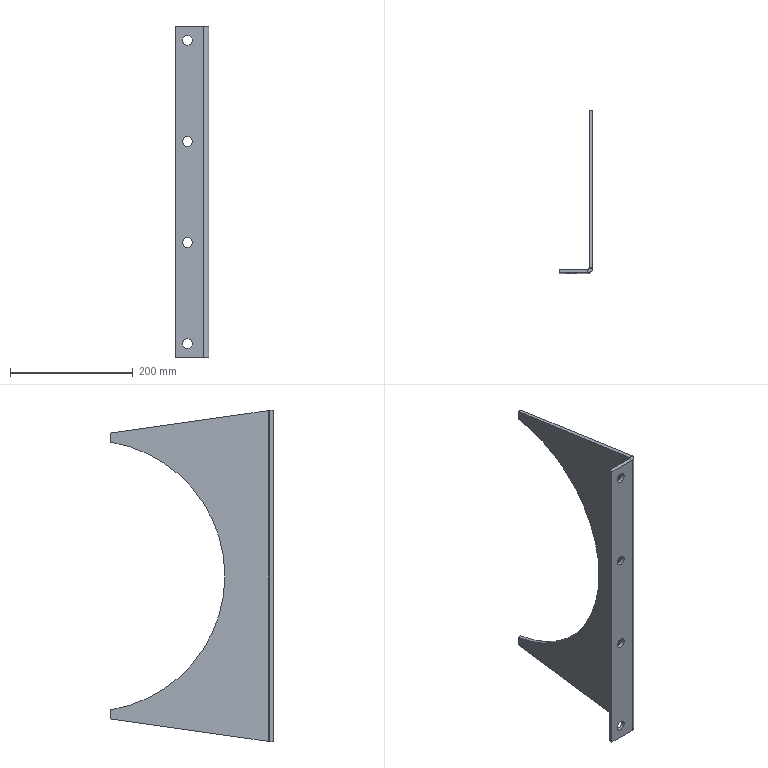Part | STEP file | Input 6 | 1 solid | 26 faces | box 55 x 265 x 540 mm | volume 579833 mm3 | plane 13 | cylinder 11 | spline 2 | commonest cylinder face diameters 16 x8 5 x1 17 x1 442 x1